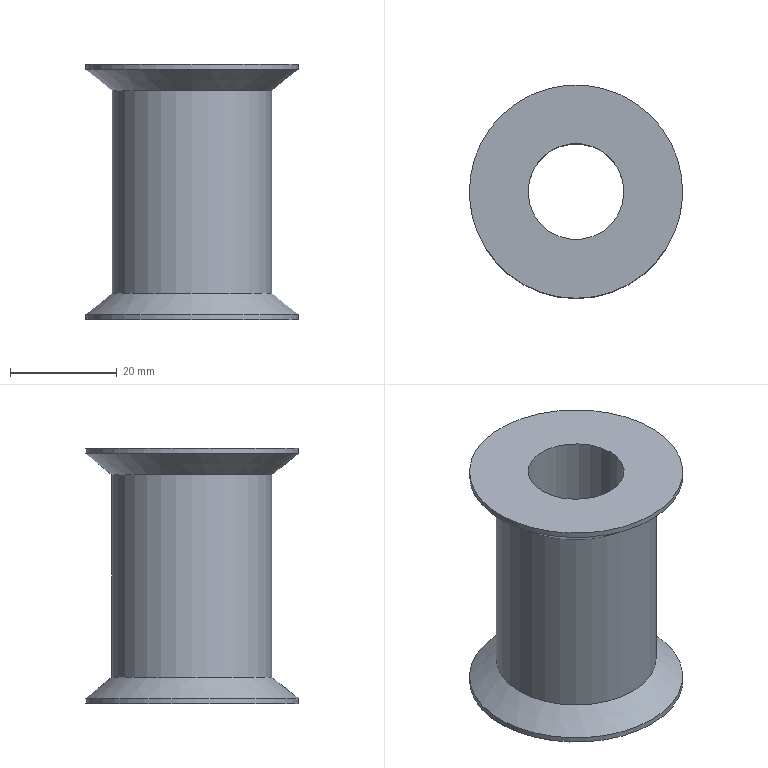Part | NX | features solid 2 | 1 solid | 8 faces | box 40 x 40 x 48 mm | volume 24909 mm3 | cylinder 4 | plane 2 | cone 2 | commonest cylinder face diameters 40 x2 18 x1 30 x1
STEP:
#1=CARTESIAN_POINT('',(-1473.255,389.161,-17.));
#2=VERTEX_POINT('',#1);
#3=CARTESIAN_POINT('',(-1473.255,409.161,-17.));
#4=DIRECTION('',(0.,0.,-1.));
#5=DIRECTION('',(0.,-1.,0.));
#6=AXIS2_PLACEMENT_3D('',#3,#4,#5);
#7=CIRCLE('',#6,20.);
#8=EDGE_CURVE('',#2,#2,#7,.T.);
#9=ORIENTED_EDGE('',*,*,#8,.T.);
#10=EDGE_LOOP('',(#9));
#11=FACE_BOUND('',#10,.T.);
#12=CARTESIAN_POINT('',(-1464.255,409.161,-17.));
#13=VERTEX_POINT('',#12);
#14=CARTESIAN_POINT('',(-1473.255,409.161,-17.));
#15=DIRECTION('',(0.,0.,-1.));
#16=DIRECTION('',(1.,0.,0.));
#17=AXIS2_PLACEMENT_3D('',#14,#15,#16);
#18=CIRCLE('',#17,9.);
#19=EDGE_CURVE('',#13,#13,#18,.F.);
#20=ORIENTED_EDGE('',*,*,#19,.T.);
#21=EDGE_LOOP('',(#20));
#22=FACE_BOUND('',#21,.T.);
#23=CARTESIAN_POINT('',(-1473.255,409.161,-17.));
#24=DIRECTION('',(0.,0.,-1.));
#25=DIRECTION('',(0.,-1.,0.));
#26=AXIS2_PLACEMENT_3D('',#23,#24,#25);
#27=PLANE('',#26);
#28=ADVANCED_FACE('',(#11,#22),#27,.T.);
#29=CARTESIAN_POINT('',(-1473.255,389.161,31.));
#30=VERTEX_POINT('',#29);
#31=CARTESIAN_POINT('',(-1473.255,409.161,31.));
#32=DIRECTION('',(0.,0.,-1.));
#33=DIRECTION('',(0.,-1.,0.));
#34=AXIS2_PLACEMENT_3D('',#31,#32,#33);
#35=CIRCLE('',#34,20.);
#36=EDGE_CURVE('',#30,#30,#35,.T.);
#37=ORIENTED_EDGE('',*,*,#36,.F.);
#38=EDGE_LOOP('',(#37));
#39=FACE_BOUND('',#38,.T.);
#40=CARTESIAN_POINT('',(-1464.255,409.161,31.));
#41=VERTEX_POINT('',#40);
#42=CARTESIAN_POINT('',(-1473.255,409.161,31.));
#43=DIRECTION('',(0.,0.,-1.));
#44=DIRECTION('',(1.,0.,0.));
#45=AXIS2_PLACEMENT_3D('',#42,#43,#44);
#46=CIRCLE('',#45,9.);
#47=EDGE_CURVE('',#41,#41,#46,.T.);
#48=ORIENTED_EDGE('',*,*,#47,.T.);
#49=EDGE_LOOP('',(#48));
#50=FACE_BOUND('',#49,.T.);
#51=CARTESIAN_POINT('',(-1473.255,409.161,31.));
#52=DIRECTION('',(0.,0.,-1.));
#53=DIRECTION('',(0.,-1.,0.));
#54=AXIS2_PLACEMENT_3D('',#51,#52,#53);
#55=PLANE('',#54);
#56=ADVANCED_FACE('',(#39,#50),#55,.F.);
#57=CARTESIAN_POINT('',(-1473.255,394.161,26.));
#58=VERTEX_POINT('',#57);
#59=CARTESIAN_POINT('',(-1473.255,409.161,26.));
#60=DIRECTION('',(0.,0.,-1.));
#61=DIRECTION('',(0.,-1.,0.));
#62=AXIS2_PLACEMENT_3D('',#59,#60,#61);
#63=CIRCLE('',#62,15.);
#64=EDGE_CURVE('',#58,#58,#63,.T.);
#65=ORIENTED_EDGE('',*,*,#64,.T.);
#66=EDGE_LOOP('',(#65));
#67=FACE_BOUND('',#66,.T.);
#68=CARTESIAN_POINT('',(-1473.255,394.161,-12.));
#69=VERTEX_POINT('',#68);
#70=CARTESIAN_POINT('',(-1473.255,409.161,-12.));
#71=DIRECTION('',(0.,0.,-1.));
#72=DIRECTION('',(0.,-1.,0.));
#73=AXIS2_PLACEMENT_3D('',#70,#71,#72);
#74=CIRCLE('',#73,15.);
#75=EDGE_CURVE('',#69,#69,#74,.F.);
#76=ORIENTED_EDGE('',*,*,#75,.T.);
#77=EDGE_LOOP('',(#76));
#78=FACE_BOUND('',#77,.T.);
#79=CARTESIAN_POINT('',(-1473.255,409.161,-17.));
#80=DIRECTION('',(0.,0.,1.));
#81=DIRECTION('',(0.,1.,0.));
#82=AXIS2_PLACEMENT_3D('',#79,#80,#81);
#83=CYLINDRICAL_SURFACE('',#82,15.);
#84=ADVANCED_FACE('',(#67,#78),#83,.T.);
#85=CARTESIAN_POINT('',(-1473.255,389.161,-16.));
#86=VERTEX_POINT('',#85);
#87=CARTESIAN_POINT('',(-1473.255,409.161,-16.));
#88=DIRECTION('',(0.,0.,-1.));
#89=DIRECTION('',(0.,-1.,0.));
#90=AXIS2_PLACEMENT_3D('',#87,#88,#89);
#91=CIRCLE('',#90,20.);
#92=EDGE_CURVE('',#86,#86,#91,.T.);
#93=ORIENTED_EDGE('',*,*,#92,.T.);
#94=EDGE_LOOP('',(#93));
#95=FACE_BOUND('',#94,.T.);
#96=ORIENTED_EDGE('',*,*,#8,.F.);
#97=EDGE_LOOP('',(#96));
#98=FACE_BOUND('',#97,.T.);
#99=CARTESIAN_POINT('',(-1473.255,409.161,-17.));
#100=DIRECTION('',(0.,0.,1.));
#101=DIRECTION('',(0.,1.,0.));
#102=AXIS2_PLACEMENT_3D('',#99,#100,#101);
#103=CYLINDRICAL_SURFACE('',#102,20.);
#104=ADVANCED_FACE('',(#95,#98),#103,.T.);
#105=ORIENTED_EDGE('',*,*,#75,.F.);
#106=EDGE_LOOP('',(#105));
#107=FACE_BOUND('',#106,.T.);
#108=ORIENTED_EDGE('',*,*,#92,.F.);
#109=EDGE_LOOP('',(#108));
#110=FACE_BOUND('',#109,.T.);
#111=CARTESIAN_POINT('',(-1473.255,409.161,-16.));
#112=DIRECTION('',(0.,0.,-1.));
#113=DIRECTION('',(0.,-1.,0.));
#114=AXIS2_PLACEMENT_3D('',#111,#112,#113);
#115=CONICAL_SURFACE('',#114,20.,0.8961);
#116=ADVANCED_FACE('',(#107,#110),#115,.T.);
#117=CARTESIAN_POINT('',(-1473.255,389.161,30.));
#118=VERTEX_POINT('',#117);
#119=CARTESIAN_POINT('',(-1473.255,409.161,30.));
#120=DIRECTION('',(0.,0.,-1.));
#121=DIRECTION('',(0.,-1.,0.));
#122=AXIS2_PLACEMENT_3D('',#119,#120,#121);
#123=CIRCLE('',#122,20.);
#124=EDGE_CURVE('',#118,#118,#123,.F.);
#125=ORIENTED_EDGE('',*,*,#124,.T.);
#126=EDGE_LOOP('',(#125));
#127=FACE_BOUND('',#126,.T.);
#128=ORIENTED_EDGE('',*,*,#36,.T.);
#129=EDGE_LOOP('',(#128));
#130=FACE_BOUND('',#129,.T.);
#131=CARTESIAN_POINT('',(-1473.255,409.161,26.));
#132=DIRECTION('',(0.,0.,1.));
#133=DIRECTION('',(0.,1.,0.));
#134=AXIS2_PLACEMENT_3D('',#131,#132,#133);
#135=CYLINDRICAL_SURFACE('',#134,20.);
#136=ADVANCED_FACE('',(#127,#130),#135,.T.);
#137=ORIENTED_EDGE('',*,*,#124,.F.);
#138=EDGE_LOOP('',(#137));
#139=FACE_BOUND('',#138,.T.);
#140=ORIENTED_EDGE('',*,*,#64,.F.);
#141=EDGE_LOOP('',(#140));
#142=FACE_BOUND('',#141,.T.);
#143=CARTESIAN_POINT('',(-1473.255,409.161,26.));
#144=DIRECTION('',(0.,0.,1.));
#145=DIRECTION('',(0.,1.,0.));
#146=AXIS2_PLACEMENT_3D('',#143,#144,#145);
#147=CONICAL_SURFACE('',#146,15.,0.8961);
#148=ADVANCED_FACE('',(#139,#142),#147,.T.);
#149=ORIENTED_EDGE('',*,*,#47,.F.);
#150=EDGE_LOOP('',(#149));
#151=FACE_BOUND('',#150,.T.);
#152=ORIENTED_EDGE('',*,*,#19,.F.);
#153=EDGE_LOOP('',(#152));
#154=FACE_BOUND('',#153,.T.);
#155=CARTESIAN_POINT('',(-1473.255,409.161,27.));
#156=DIRECTION('',(0.,0.,1.));
#157=DIRECTION('',(0.,1.,0.));
#158=AXIS2_PLACEMENT_3D('',#155,#156,#157);
#159=CYLINDRICAL_SURFACE('',#158,9.);
#160=ADVANCED_FACE('',(#151,#154),#159,.F.);
#161=CLOSED_SHELL('',(#28,#56,#84,#104,#116,#136,#148,#160));
#162=MANIFOLD_SOLID_BREP('',#161);
#163=(LENGTH_UNIT()NAMED_UNIT(*)SI_UNIT(.MILLI.,.METRE.));
#164=UNCERTAINTY_MEASURE_WITH_UNIT(LENGTH_MEASURE(0.00001),#163,'','');
#165=(NAMED_UNIT(*)PLANE_ANGLE_UNIT()SI_UNIT($,.RADIAN.));
#166=(NAMED_UNIT(*)SI_UNIT($,.STERADIAN.)SOLID_ANGLE_UNIT());
#167=(GEOMETRIC_REPRESENTATION_CONTEXT(3)GLOBAL_UNCERTAINTY_ASSIGNED_CONTEXT((#164))GLOBAL_UNIT_ASSIGNED_CONTEXT((#163,#165,#166))REPRESENTATION_CONTEXT('',''));
#168=ADVANCED_BREP_SHAPE_REPRESENTATION('',(#162),#167);